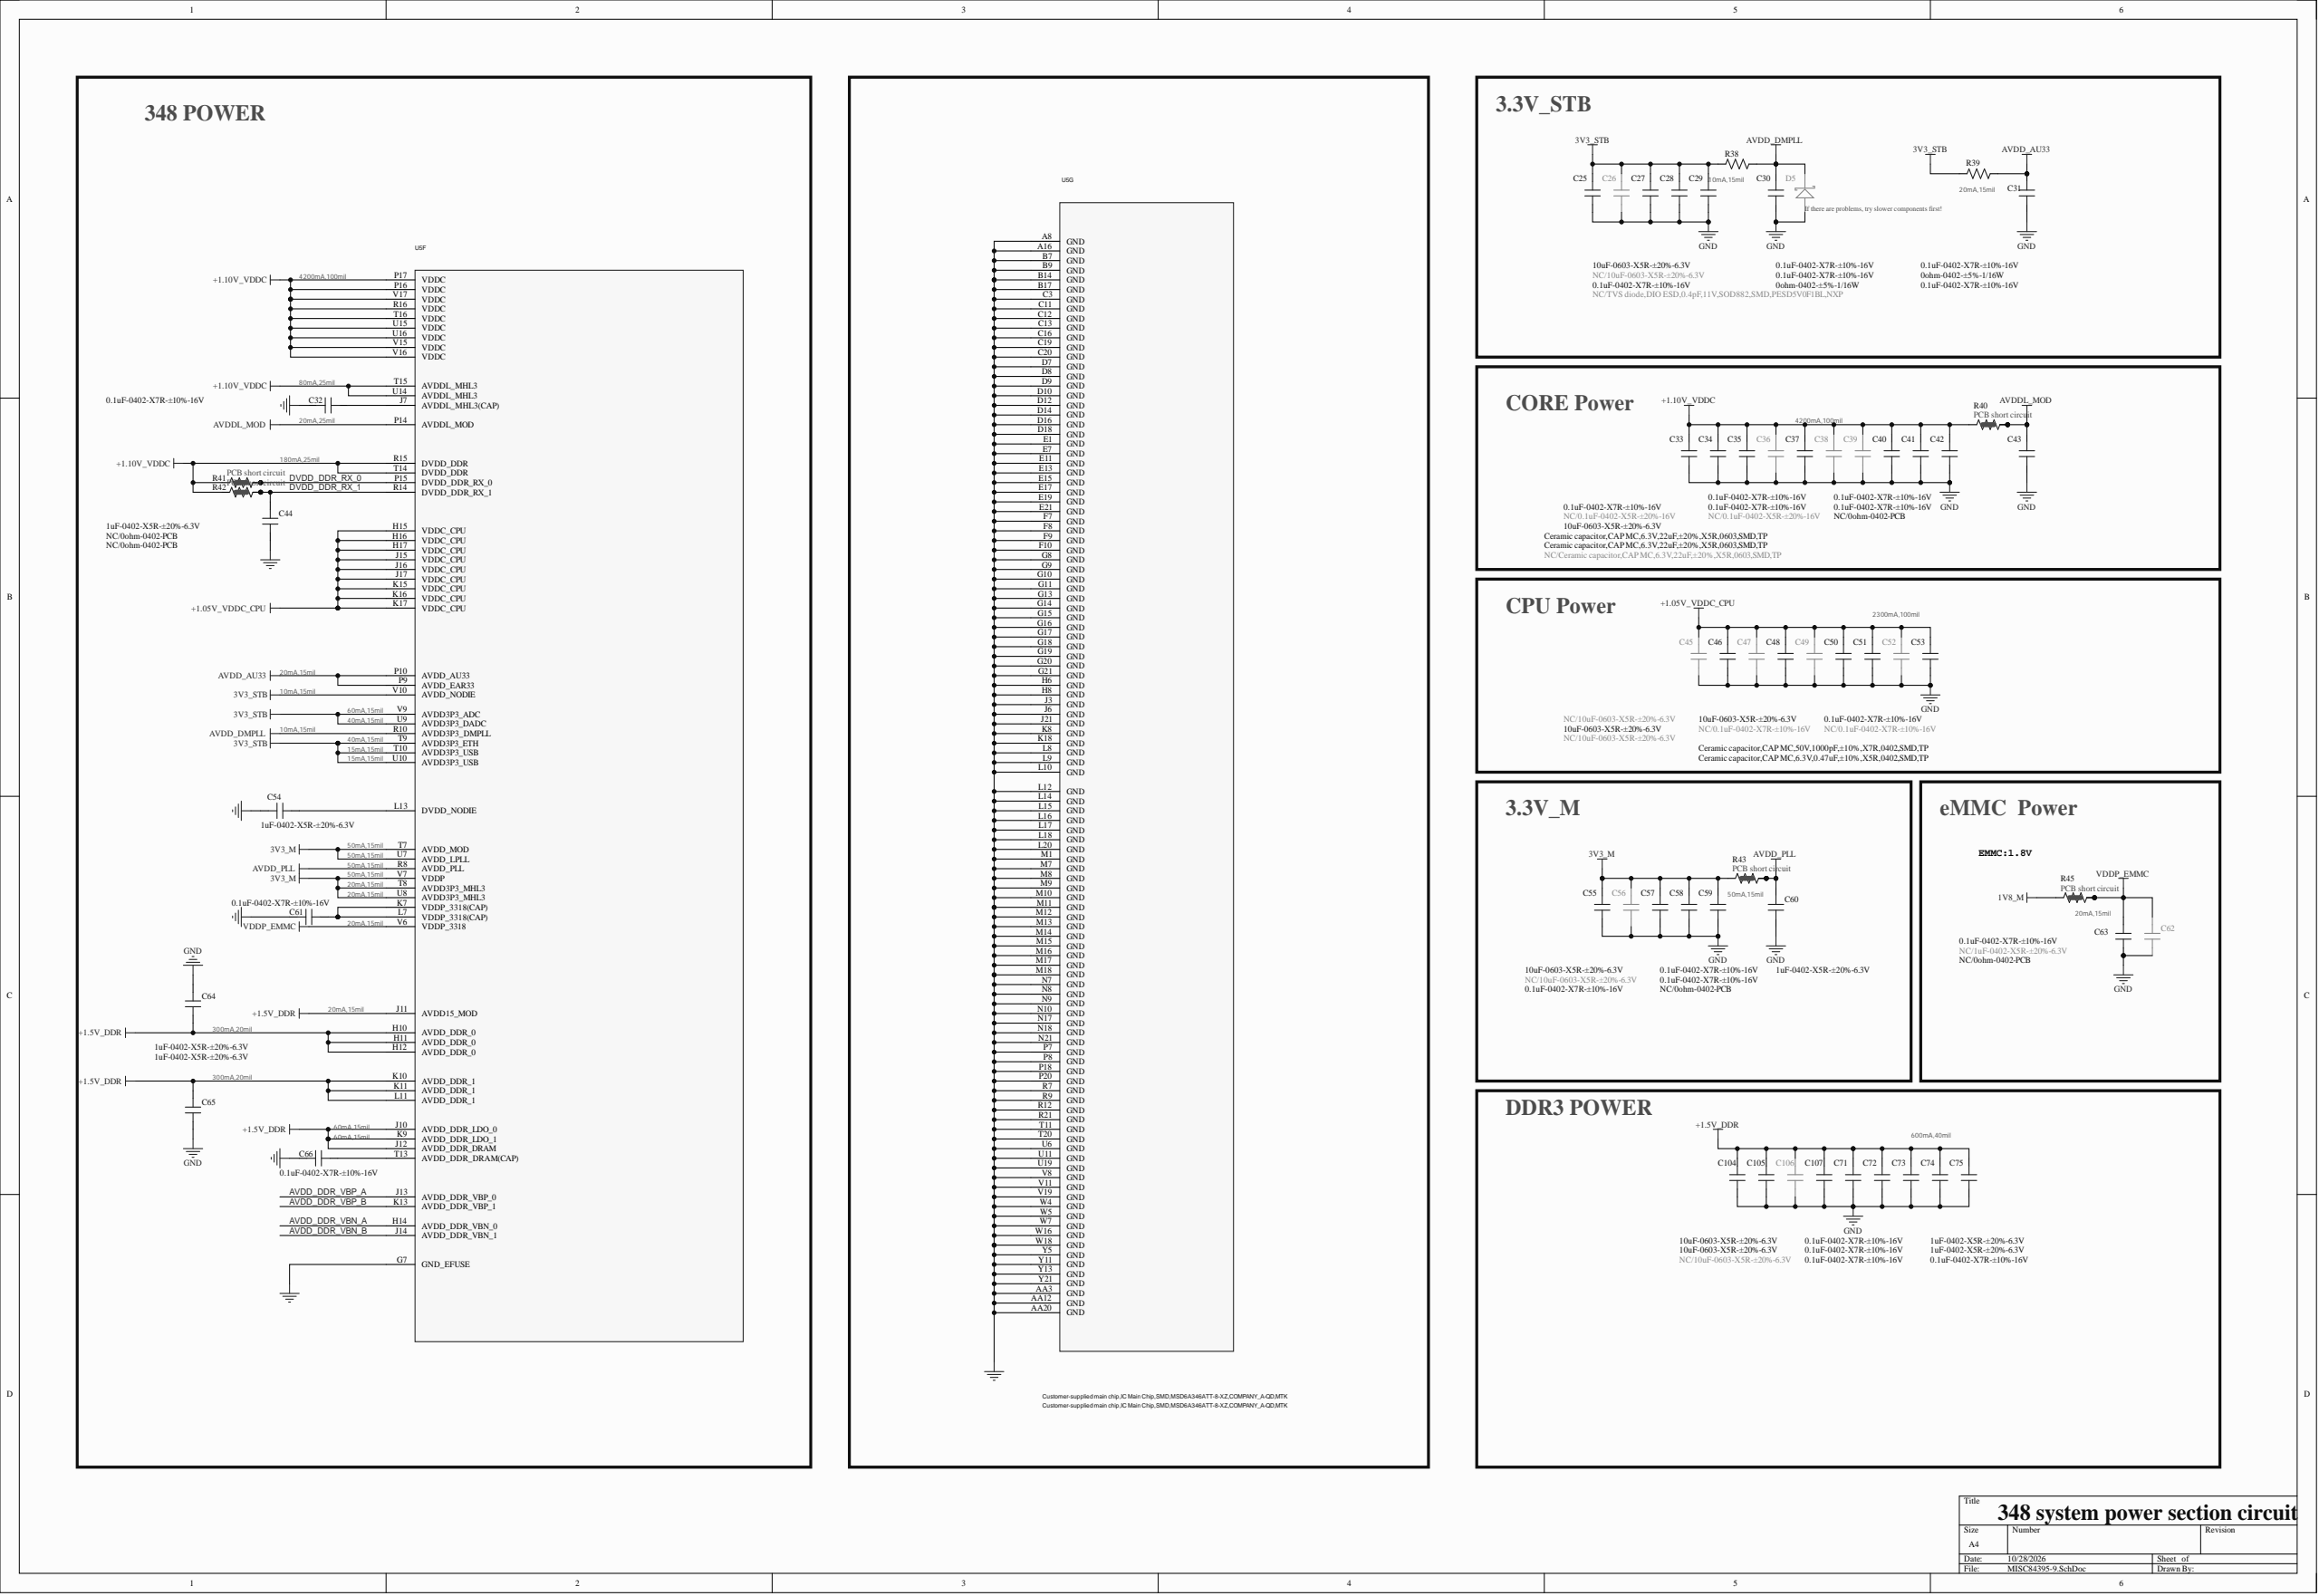Circuit board | Altium Designer | 951 parts | 509 nets | one sheet of the schematic
Parts on this sheet (reference | value | footprint):
C25 | 10uF-0603-X5R-±20%-6.3V | C0603
C26 | NC/10uF-0603-X5R-±20%-6.3V | C0603
C27 | 0.1uF-0402-X7R-±10%-16V | C0402
C28 | 0.1uF-0402-X7R-±10%-16V | C0402
C29 | 0.1uF-0402-X7R-±10%-16V | C0402
C30 | 0.1uF-0402-X7R-±10%-16V | C0402
C31 | 0.1uF-0402-X7R-±10%-16V | C0402
C32 | 0.1uF-0402-X7R-±10%-16V | C0402
C33 | 10uF-0603-X5R-±20%-6.3V | C0603
C34 | Ceramic capacitor,CAP MC,6.3V,22uF,±20%,X5R,0603,SMD,TP | C0603
C35 | Ceramic capacitor,CAP MC,6.3V,22uF,±20%,X5R,0603,SMD,TP | C0603
C36 | NC/Ceramic capacitor,CAP MC,6.3V,22uF,±20%,X5R,0603,SMD,TP | C0603
C37 | 0.1uF-0402-X7R-±10%-16V | C0402
C38 | NC/0.1uF-0402-X5R-±20%-16V | C0402
C39 | NC/0.1uF-0402-X5R-±20%-16V | C0402
C40 | 0.1uF-0402-X7R-±10%-16V | C0402
C41 | 0.1uF-0402-X7R-±10%-16V | C0402
C42 | 0.1uF-0402-X7R-±10%-16V | C0402
C43 | 0.1uF-0402-X7R-±10%-16V | C0402
C44 | 1uF-0402-X5R-±20%-6.3V | C0402
C45 | NC/10uF-0603-X5R-±20%-6.3V | C0603
C46 | 10uF-0603-X5R-±20%-6.3V | C0603
C47 | NC/10uF-0603-X5R-±20%-6.3V | C0603
C48 | 10uF-0603-X5R-±20%-6.3V | C0603
C49 | NC/0.1uF-0402-X7R-±10%-16V | C0402
C50 | Ceramic capacitor,CAP MC,50V,1000pF,±10%,X7R,0402,SMD,TP | C0402
C51 | 0.1uF-0402-X7R-±10%-16V | C0402
C52 | NC/0.1uF-0402-X7R-±10%-16V | C0402
C53 | Ceramic capacitor,CAP MC,6.3V,0.47uF,±10%,X5R,0402,SMD,TP | C0402
C54 | 1uF-0402-X5R-±20%-6.3V | C0402
C55 | 10uF-0603-X5R-±20%-6.3V | C0603
C56 | NC/10uF-0603-X5R-±20%-6.3V | C0603
C57 | 0.1uF-0402-X7R-±10%-16V | C0402
C58 | 0.1uF-0402-X7R-±10%-16V | C0402
C59 | 0.1uF-0402-X7R-±10%-16V | C0402
C60 | 1uF-0402-X5R-±20%-6.3V | C0402
C61 | 0.1uF-0402-X7R-±10%-16V | C0402
C62 | NC/1uF-0402-X5R-±20%-6.3V | C0402
C63 | 0.1uF-0402-X7R-±10%-16V | C0402
C64 | 1uF-0402-X5R-±20%-6.3V | C0402
C65 | 1uF-0402-X5R-±20%-6.3V | C0402
C66 | 0.1uF-0402-X7R-±10%-16V | C0402
C71 | 0.1uF-0402-X7R-±10%-16V | C0402
C72 | 0.1uF-0402-X7R-±10%-16V | C0402
C73 | 0.1uF-0402-X7R-±10%-16V | C0402
C74 | 1uF-0402-X5R-±20%-6.3V | C0402
C75 | 1uF-0402-X5R-±20%-6.3V | C0402
C104 | 10uF-0603-X5R-±20%-6.3V | C0603
C105 | 10uF-0603-X5R-±20%-6.3V | C0603
C106 | NC/10uF-0603-X5R-±20%-6.3V | C0603
C107 | 0.1uF-0402-X7R-±10%-16V | C0402
D5 | NC/TVS diode,DIO ESD,0.4pF,11V,SOD882,SMD,PESD5V0F1BL,NXP | DIODE-S0402
R38 | 0ohm-0402-±5%-1/16W | R0402
R39 | 0ohm-0402-±5%-1/16W | R0402
R40 | NC/0ohm-0402-PCB | R0402SC
R41 | NC/0ohm-0402-PCB | R0402SC
R42 | NC/0ohm-0402-PCB | R0402SC
R43 | NC/0ohm-0402-PCB | R0402SC
R45 | NC/0ohm-0402-PCB | R0402SC
U5 | Customer-supplied main chip,IC Main Chip,SMD,MSD6A346ATT-8-XZ,COMPANY_A-QD,MTK | BGA406/0.8
Nets of these parts (net: part-pin ...):
VDDP_EMMC: C62-2 C63-2 R45-2 R45-3 U5-V6
NetC66_1: C66-1 U5-T13
NetC61_2: C61-2 U5-K7 U5-L7
NetC54_1: C54-1 U5-L13
NetC32_2: C32-2 U5-J7
GND: C25-1 C26-1 C27-1 C28-1 C29-1 C30-1 C31-1 C32-1 C33-1 C34-1 C35-1 C36-1 C37-1 C38-1 C39-1 C40-1 C41-1 C42-1 C43-1 C44-1 C45-1 C46-1 C47-1 C48-1 C49-1 C50-1 C51-1 C52-1 C53-1 C54-2 C55-1 C56-1 C57-1 C58-1 C59-1 C60-1 C61-1 C62-1 C63-1 C64-2 C65-1 C66-2 C71-1 C72-1 C73-1 C74-1 C75-1 C104-1 C105-1 C106-1 C107-1 D5-A U5-A8 U5-A16 U5-AA3 U5-AA12 U5-AA20 U5-B7 U5-B9 U5-B14 U5-B17 U5-C3 U5-C11 U5-C12 U5-C13 U5-C16 U5-C19 U5-C20 U5-D7 U5-D8 U5-D9 U5-D10 U5-D12 U5-D14 U5-D16 U5-D18 U5-E1 U5-E7 U5-E11 U5-E13 U5-E15 U5-E17 U5-E19 U5-E21 U5-F7 U5-F8 U5-F9 U5-F10 U5-G7 U5-G8 U5-G9 U5-G10 U5-G11 U5-G13 U5-G14 U5-G15 U5-G16 U5-G17 U5-G18 U5-G19 U5-G20 U5-G21 U5-H6 U5-H8 U5-J3 U5-J6 U5-J21 U5-K8 U5-K18 U5-L8 U5-L9 U5-L10 U5-L12 U5-L14 U5-L15 U5-L16 U5-L17 U5-L18 U5-L20 U5-M1 U5-M7 U5-M8 U5-M9 U5-M10 U5-M11 U5-M12 U5-M13 U5-M14 U5-M15 U5-M16 U5-M17 U5-M18 U5-N7 U5-N8 U5-N9 U5-N10 U5-N17 U5-N18 U5-N21 U5-P7 U5-P8 U5-P18 U5-P20 U5-R7 U5-R9 U5-R12 U5-R21 U5-T11 U5-T20 U5-U6 U5-U11 U5-U19 U5-V8 U5-V11 U5-V19 U5-W4 U5-W5 U5-W7 U5-W16 U5-W18 U5-Y5 U5-Y11 U5-Y13 U5-Y21
DVDD_DDR_RX_1: C44-2 R42-2 R42-3 U5-R14
DVDD_DDR_RX_0: R41-2 R41-3 U5-P15
AVDDL_MOD: C43-2 R40-2 R40-3 U5-P14
AVDD_PLL: C60-2 R43-2 R43-3 U5-R8
AVDD_DMPLL: C30-2 D5-K R38-2 U5-R10
AVDD_AU33: C31-2 R39-2 U5-P9 U5-P10
+1.10V_VDDC: C33-2 C34-2 C35-2 C36-2 C37-2 C38-2 C39-2 C40-2 C41-2 C42-2 R40-1 R41-1 R42-1 U5-P16 U5-P17 U5-R15 U5-R16 U5-T14 U5-T15 U5-T16 U5-U14 U5-U15 U5-U16 U5-V15 U5-V16 U5-V17
+1.05V_VDDC_CPU: C45-2 C46-2 C47-2 C48-2 C49-2 C50-2 C51-2 C52-2 C53-2 U5-H15 U5-H16 U5-H17 U5-J15 U5-J16 U5-J17 U5-K15 U5-K16 U5-K17
+1.5V_DDR: C64-1 C65-2 C71-2 C72-2 C73-2 C74-2 C75-2 C104-2 C105-2 C106-2 C107-2 U5-H10 U5-H11 U5-H12 U5-J10 U5-J11 U5-J12 U5-K9 U5-K10 U5-K11 U5-L11
3V3_STB: C25-2 C26-2 C27-2 C28-2 C29-2 R38-1 R39-1 U5-T9 U5-T10 U5-U9 U5-U10 U5-V9 U5-V10
3V3_M: C55-2 C56-2 C57-2 C58-2 C59-2 R43-1 U5-T7 U5-T8 U5-U7 U5-U8 U5-V7
1V8_M: R45-1